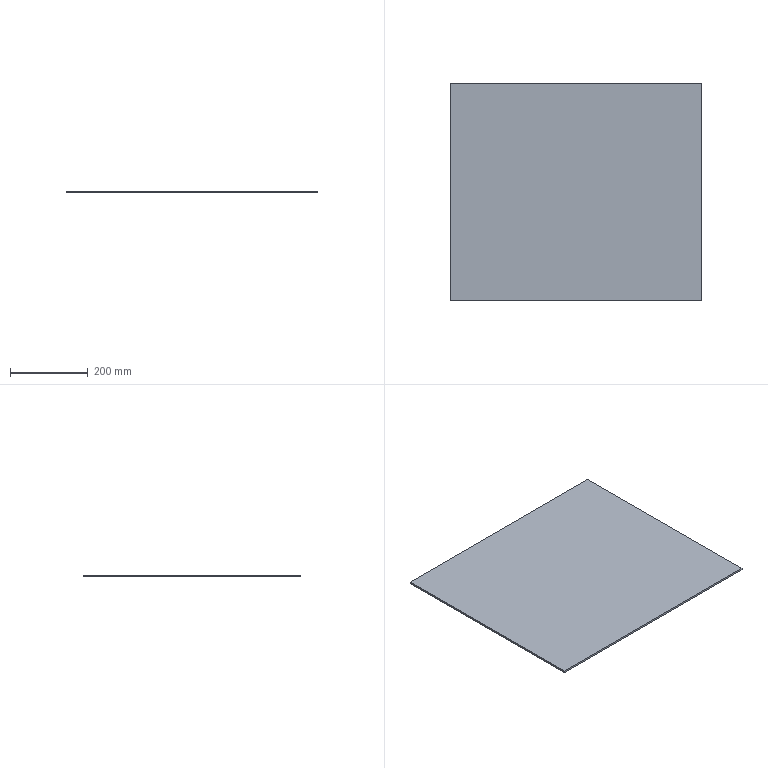Part | SolidWorks | features BaseBody 1, ICE 1 | 1 solid | 6 faces | box 647 x 560 x 5 mm | volume 1811600 mm3 | plane 6
STEP:
#1=CARTESIAN_POINT('',(87.,600.,-395.));
#2=VERTEX_POINT('',#1);
#3=CARTESIAN_POINT('',(87.,40.,-395.));
#4=VERTEX_POINT('',#3);
#5=CARTESIAN_POINT('',(87.,600.,-395.));
#6=DIRECTION('',(0.,-1.,0.));
#7=VECTOR('',#6,1000.);
#8=LINE('',#5,#7);
#9=EDGE_CURVE('',#2,#4,#8,.T.);
#10=ORIENTED_EDGE('',*,*,#9,.F.);
#11=CARTESIAN_POINT('',(-560.,600.,-395.));
#12=VERTEX_POINT('',#11);
#13=CARTESIAN_POINT('',(-560.,600.,-395.));
#14=DIRECTION('',(1.,0.,0.));
#15=VECTOR('',#14,1000.);
#16=LINE('',#13,#15);
#17=EDGE_CURVE('',#12,#2,#16,.T.);
#18=ORIENTED_EDGE('',*,*,#17,.F.);
#19=CARTESIAN_POINT('',(-560.,40.,-395.));
#20=VERTEX_POINT('',#19);
#21=CARTESIAN_POINT('',(-560.,40.,-395.));
#22=DIRECTION('',(0.,1.,0.));
#23=VECTOR('',#22,1000.);
#24=LINE('',#21,#23);
#25=EDGE_CURVE('',#20,#12,#24,.T.);
#26=ORIENTED_EDGE('',*,*,#25,.F.);
#27=CARTESIAN_POINT('',(560.,40.,-395.));
#28=DIRECTION('',(-1.,0.,0.));
#29=VECTOR('',#28,1000.);
#30=LINE('',#27,#29);
#31=EDGE_CURVE('',#4,#20,#30,.T.);
#32=ORIENTED_EDGE('',*,*,#31,.F.);
#33=EDGE_LOOP('',(#10,#18,#26,#32));
#34=FACE_OUTER_BOUND('',#33,.T.);
#35=CARTESIAN_POINT('',(0.,320.,-395.));
#36=DIRECTION('',(0.,0.,1.));
#37=DIRECTION('',(1.,0.,0.));
#38=AXIS2_PLACEMENT_3D('',#35,#36,#37);
#39=PLANE('',#38);
#40=ADVANCED_FACE('',(#34),#39,.T.);
#41=CARTESIAN_POINT('',(87.,40.,-400.));
#42=VERTEX_POINT('',#41);
#43=CARTESIAN_POINT('',(87.,600.,-400.));
#44=VERTEX_POINT('',#43);
#45=CARTESIAN_POINT('',(87.,320.,-400.));
#46=DIRECTION('',(0.,1.,0.));
#47=VECTOR('',#46,1000.);
#48=LINE('',#45,#47);
#49=EDGE_CURVE('',#42,#44,#48,.T.);
#50=ORIENTED_EDGE('',*,*,#49,.F.);
#51=CARTESIAN_POINT('',(-560.,40.,-400.));
#52=VERTEX_POINT('',#51);
#53=CARTESIAN_POINT('',(-560.,40.,-400.));
#54=DIRECTION('',(1.,0.,0.));
#55=VECTOR('',#54,1000.);
#56=LINE('',#53,#55);
#57=EDGE_CURVE('',#52,#42,#56,.T.);
#58=ORIENTED_EDGE('',*,*,#57,.F.);
#59=CARTESIAN_POINT('',(-560.,600.,-400.));
#60=VERTEX_POINT('',#59);
#61=CARTESIAN_POINT('',(-560.,600.,-400.));
#62=DIRECTION('',(0.,-1.,0.));
#63=VECTOR('',#62,1000.);
#64=LINE('',#61,#63);
#65=EDGE_CURVE('',#60,#52,#64,.T.);
#66=ORIENTED_EDGE('',*,*,#65,.F.);
#67=CARTESIAN_POINT('',(560.,600.,-400.));
#68=DIRECTION('',(-1.,0.,0.));
#69=VECTOR('',#68,1000.);
#70=LINE('',#67,#69);
#71=EDGE_CURVE('',#44,#60,#70,.T.);
#72=ORIENTED_EDGE('',*,*,#71,.F.);
#73=EDGE_LOOP('',(#50,#58,#66,#72));
#74=FACE_OUTER_BOUND('',#73,.T.);
#75=CARTESIAN_POINT('',(0.,320.,-400.));
#76=DIRECTION('',(0.,0.,-1.));
#77=DIRECTION('',(0.,-1.,0.));
#78=AXIS2_PLACEMENT_3D('',#75,#76,#77);
#79=PLANE('',#78);
#80=ADVANCED_FACE('',(#74),#79,.T.);
#81=CARTESIAN_POINT('',(87.,40.,-405.));
#82=DIRECTION('',(0.,0.,1.));
#83=VECTOR('',#82,1000.);
#84=LINE('',#81,#83);
#85=EDGE_CURVE('',#42,#4,#84,.T.);
#86=ORIENTED_EDGE('',*,*,#85,.T.);
#87=ORIENTED_EDGE('',*,*,#31,.T.);
#88=CARTESIAN_POINT('',(-560.,40.,-400.));
#89=DIRECTION('',(0.,0.,1.));
#90=VECTOR('',#89,1000.);
#91=LINE('',#88,#90);
#92=EDGE_CURVE('',#52,#20,#91,.T.);
#93=ORIENTED_EDGE('',*,*,#92,.F.);
#94=ORIENTED_EDGE('',*,*,#57,.T.);
#95=EDGE_LOOP('',(#86,#87,#93,#94));
#96=FACE_OUTER_BOUND('',#95,.T.);
#97=CARTESIAN_POINT('',(-560.,40.,-400.));
#98=DIRECTION('',(0.,-1.,0.));
#99=DIRECTION('',(0.,0.,-1.));
#100=AXIS2_PLACEMENT_3D('',#97,#98,#99);
#101=PLANE('',#100);
#102=ADVANCED_FACE('',(#96),#101,.T.);
#103=CARTESIAN_POINT('',(87.,600.,-400.));
#104=DIRECTION('',(0.,0.,1.));
#105=VECTOR('',#104,1000.);
#106=LINE('',#103,#105);
#107=EDGE_CURVE('',#44,#2,#106,.T.);
#108=ORIENTED_EDGE('',*,*,#107,.F.);
#109=ORIENTED_EDGE('',*,*,#71,.T.);
#110=CARTESIAN_POINT('',(-560.,600.,-395.));
#111=DIRECTION('',(0.,0.,-1.));
#112=VECTOR('',#111,1000.);
#113=LINE('',#110,#112);
#114=EDGE_CURVE('',#12,#60,#113,.T.);
#115=ORIENTED_EDGE('',*,*,#114,.F.);
#116=ORIENTED_EDGE('',*,*,#17,.T.);
#117=EDGE_LOOP('',(#108,#109,#115,#116));
#118=FACE_OUTER_BOUND('',#117,.T.);
#119=CARTESIAN_POINT('',(560.,600.,-400.));
#120=DIRECTION('',(0.,1.,0.));
#121=DIRECTION('',(1.,0.,0.));
#122=AXIS2_PLACEMENT_3D('',#119,#120,#121);
#123=PLANE('',#122);
#124=ADVANCED_FACE('',(#118),#123,.T.);
#125=ORIENTED_EDGE('',*,*,#65,.T.);
#126=ORIENTED_EDGE('',*,*,#92,.T.);
#127=ORIENTED_EDGE('',*,*,#25,.T.);
#128=ORIENTED_EDGE('',*,*,#114,.T.);
#129=EDGE_LOOP('',(#125,#126,#127,#128));
#130=FACE_OUTER_BOUND('',#129,.T.);
#131=CARTESIAN_POINT('',(-560.,600.,-400.));
#132=DIRECTION('',(-1.,0.,0.));
#133=DIRECTION('',(0.,0.,1.));
#134=AXIS2_PLACEMENT_3D('',#131,#132,#133);
#135=PLANE('',#134);
#136=ADVANCED_FACE('',(#130),#135,.T.);
#137=ORIENTED_EDGE('',*,*,#49,.T.);
#138=ORIENTED_EDGE('',*,*,#107,.T.);
#139=ORIENTED_EDGE('',*,*,#9,.T.);
#140=ORIENTED_EDGE('',*,*,#85,.F.);
#141=EDGE_LOOP('',(#137,#138,#139,#140));
#142=FACE_OUTER_BOUND('',#141,.T.);
#143=CARTESIAN_POINT('',(87.,600.,-405.));
#144=DIRECTION('',(-1.,0.,0.));
#145=DIRECTION('',(0.,0.,1.));
#146=AXIS2_PLACEMENT_3D('',#143,#144,#145);
#147=PLANE('',#146);
#148=ADVANCED_FACE('',(#142),#147,.F.);
#149=CLOSED_SHELL('',(#40,#80,#102,#124,#136,#148));
#150=MANIFOLD_SOLID_BREP('',#149);
#151=CARTESIAN_POINT('',(0.,0.,0.));
#152=DIRECTION('',(0.,0.,1.));
#153=DIRECTION('',(1.,0.,0.));
#154=AXIS2_PLACEMENT_3D('',#151,#152,#153);
#155=(LENGTH_UNIT()NAMED_UNIT(*)SI_UNIT(.MILLI.,.METRE.));
#156=UNCERTAINTY_MEASURE_WITH_UNIT(LENGTH_MEASURE(0.00001),#155,'','');
#157=(NAMED_UNIT(*)PLANE_ANGLE_UNIT()SI_UNIT($,.RADIAN.));
#158=(NAMED_UNIT(*)SI_UNIT($,.STERADIAN.)SOLID_ANGLE_UNIT());
#159=(GEOMETRIC_REPRESENTATION_CONTEXT(3)GLOBAL_UNCERTAINTY_ASSIGNED_CONTEXT((#156))GLOBAL_UNIT_ASSIGNED_CONTEXT((#155,#157,#158))REPRESENTATION_CONTEXT('',''));
#160=ADVANCED_BREP_SHAPE_REPRESENTATION('',(#150,#154),#159);